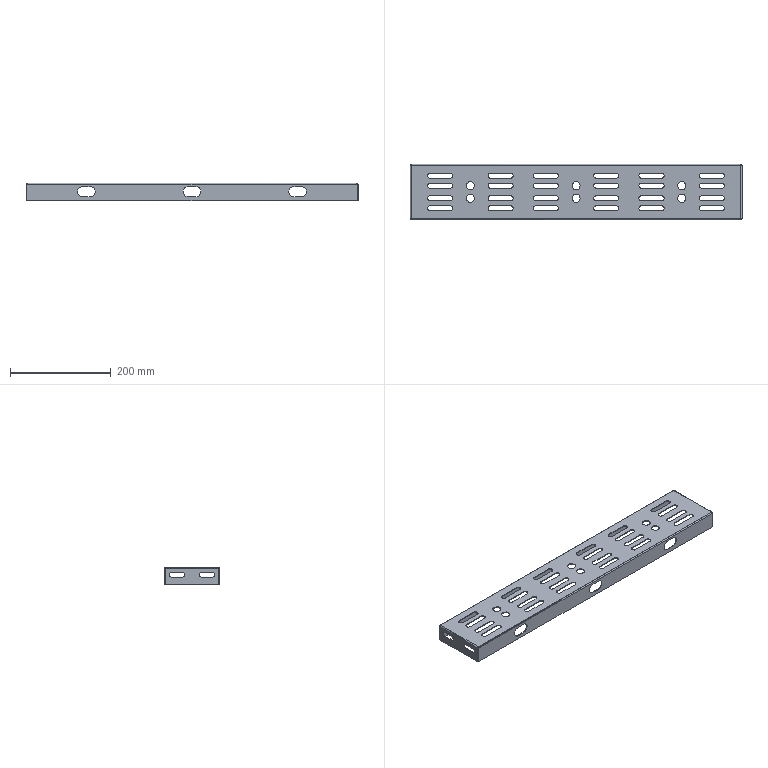Part | STEP file | Channel plate (instrument transformer) | 1 solid | 210 faces | box 659.8 x 110 x 35 mm | volume 157796 mm3 | cylinder 112 | plane 90 | spline 8 | commonest cylinder face diameters 10 x80 16 x12 20 x12 1.473 x4 4.473 x4